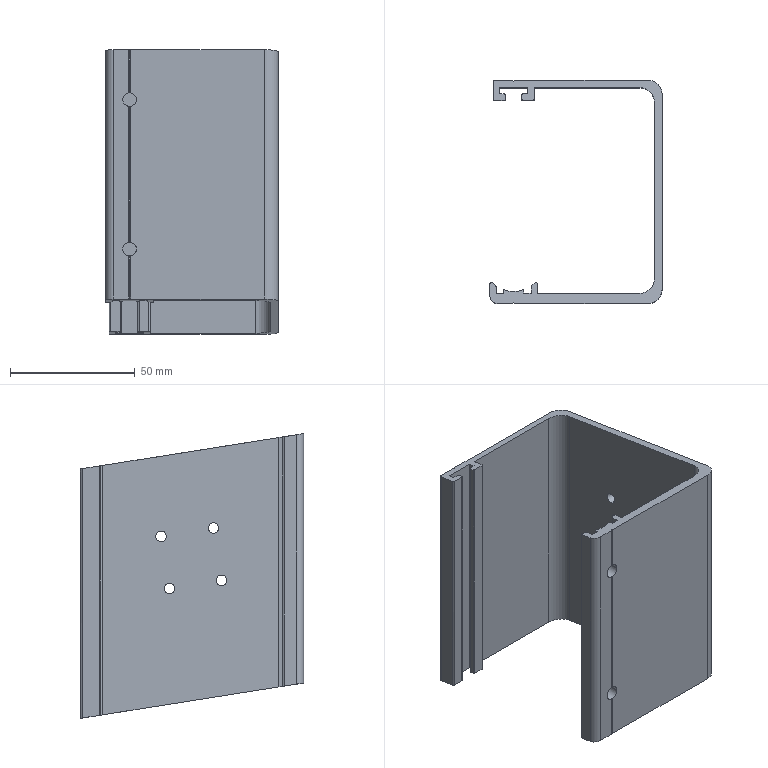Part | STEP file | 31E-01002XJ15 | 1 solid | 78 faces | box 69 x 89.5 x 114.175 mm | volume 78639 mm3 | plane 41 | cylinder 37 | commonest cylinder face diameters 1 x10 4.2 x8 3.2 x4 5.5 x4 25.4 x3 0.4 x2